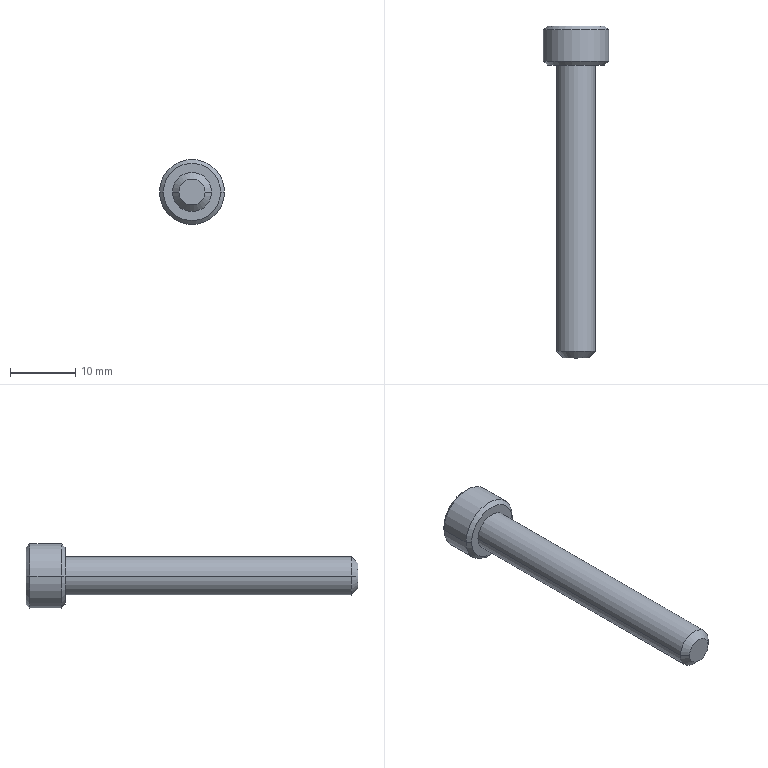Part | STEP file | BB62-M6-45L | 1 solid | 27 faces | box 10 x 51 x 10 mm | volume 1646 mm3 | plane 15 | cone 8 | cylinder 4 | commonest cylinder face diameters 6 x2 10 x2